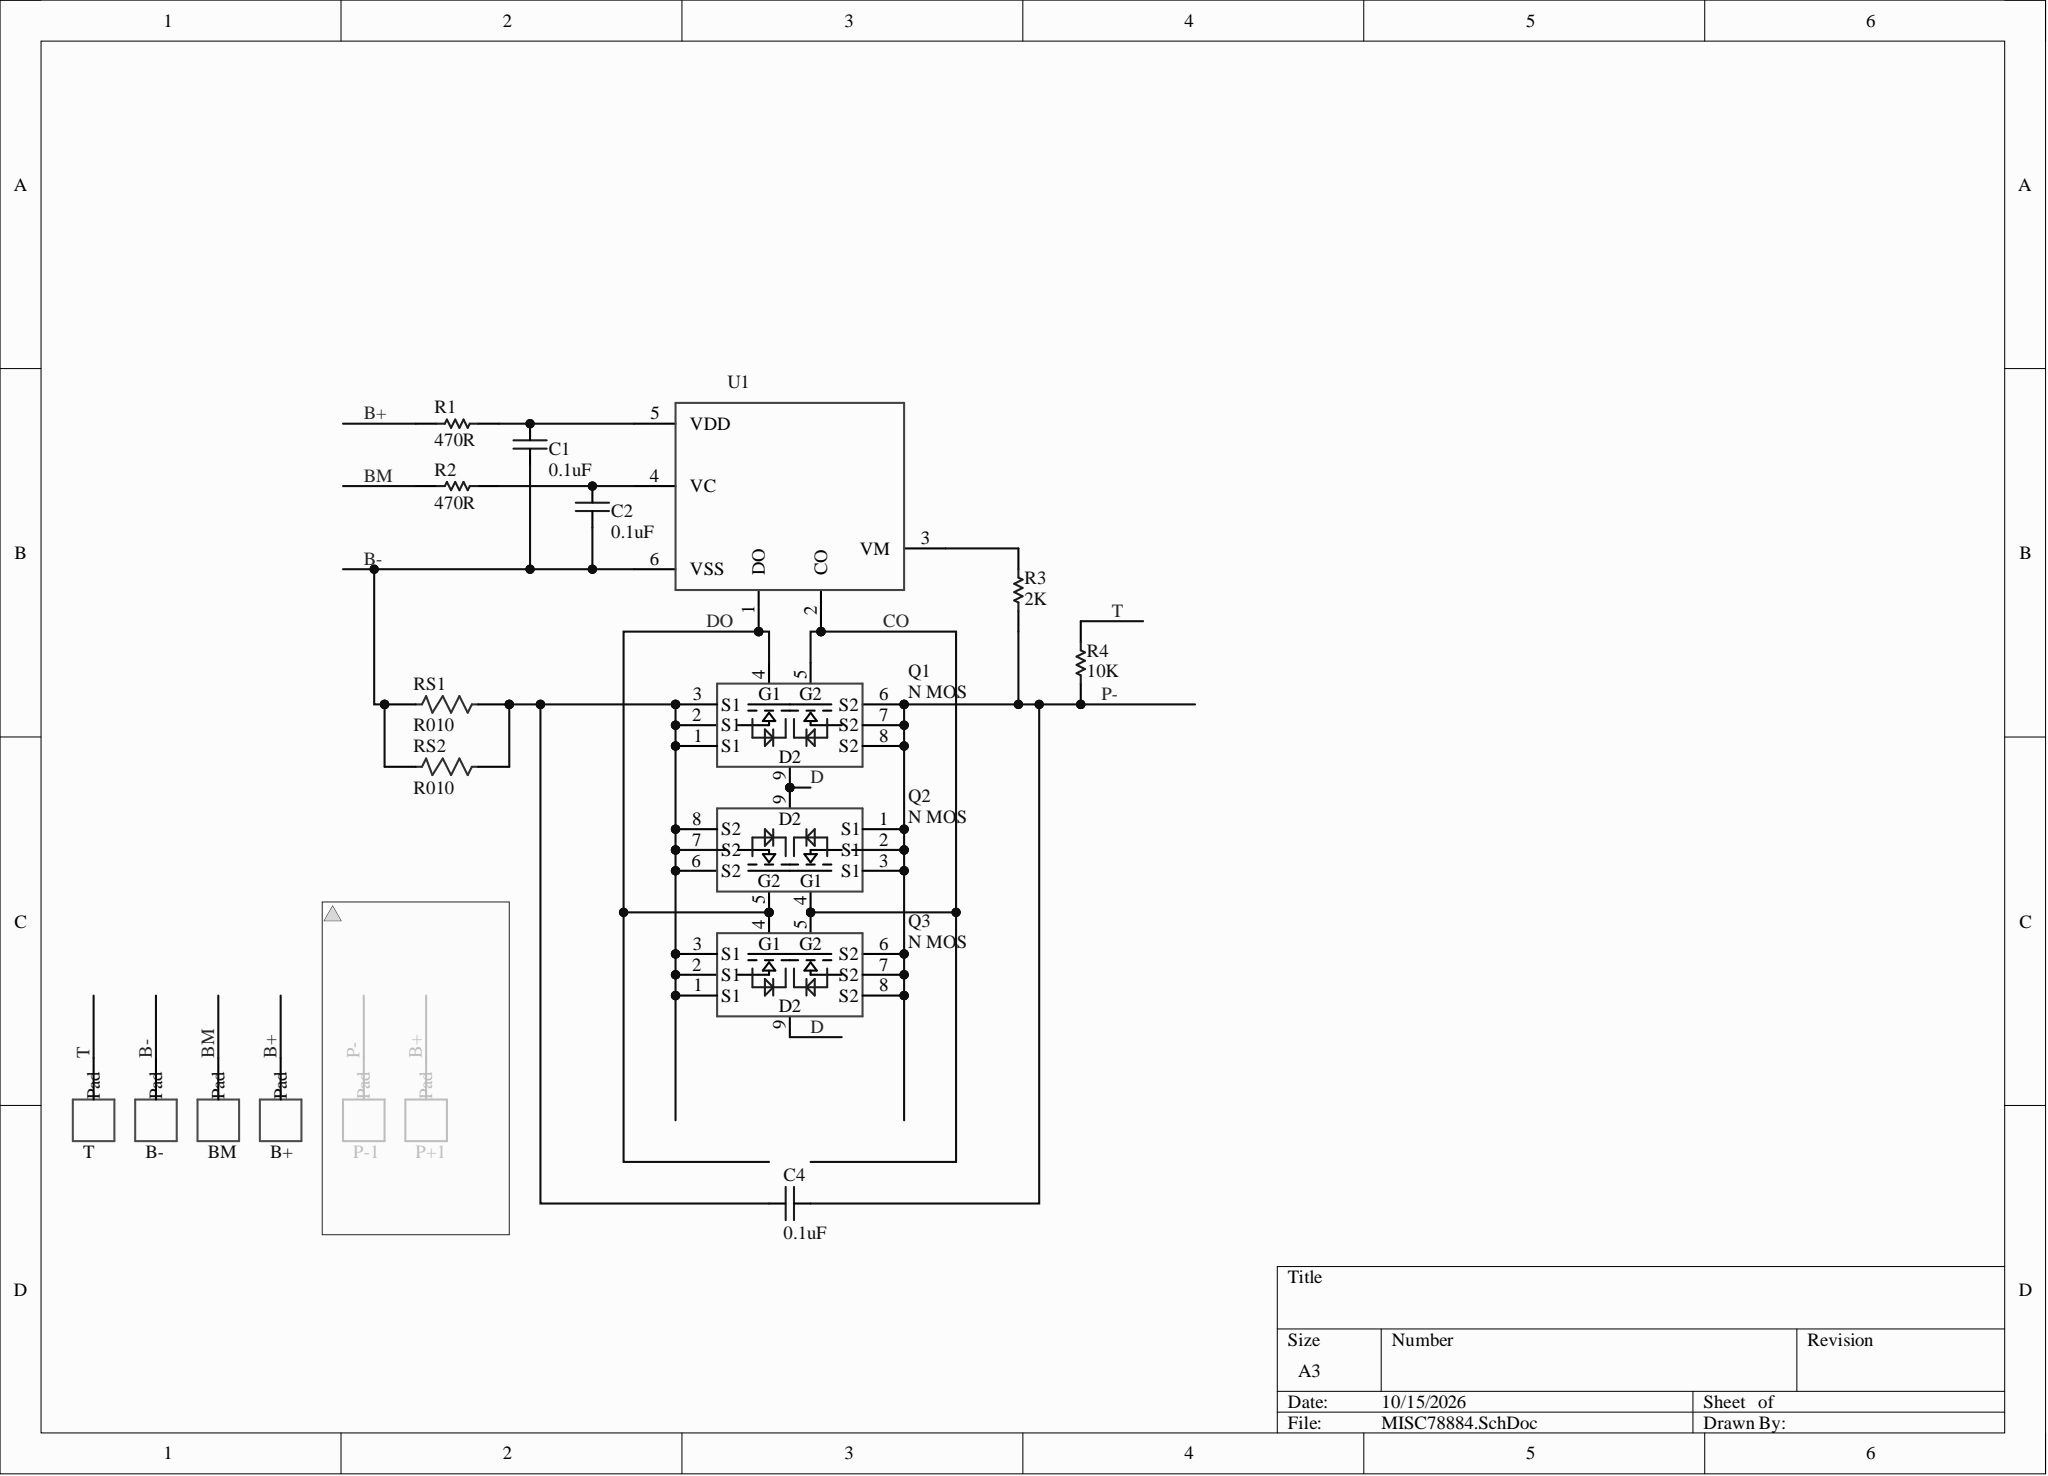Circuit board | Altium Designer | 17 parts | 12 nets
Bill of materials:
Comment,Description,Designator,Footprint,LibRef,Quantity
"Pad","Connection pad (non-through-hole)","B-, B+, BM, T","Pad10X8mm","Pad","4"
"0.1uF","SMD capacitor","C1, C2, C4","C0402A","CAP","3"
"N MOS","SMD MOS-TSSOP-8","Q1, Q2, Q3","DFN3*3-L8(2N)","2N MOS","3"
"470R","SMD resistor","R1, R2","R0402A","RES","2"
"2K","SMD resistor","R3","R0402A","RES","1"
"10K","SMD resistor","R4","R0402A","RES","1"
"R010","SMD alloy resistor","RS1, RS2","R2512L","RES2","2"
"","","U1","SOT23-6A","S-8252","1"
Netlist (Protel format):
[
B+
Pad10X8mm
Pad



]
[
B-
Pad10X8mm
Pad



]
[
BM
Pad10X8mm
Pad



]
[
C1
C0402A
0.1uF



]
[
C2
C0402A
0.1uF



]
[
C4
C0402A
0.1uF



]
[
Q1
DFN3*3-L8(2N)
N MOS



]
[
Q2
DFN3*3-L8(2N)
N MOS



]
[
Q3
DFN3*3-L8(2N)
N MOS



]
[
R1
R0402A
470R



]
[
R2
R0402A
470R



]
[
R3
R0402A
2K



]
[
R4
R0402A
10K



]
[
RS1
R2512L
R010



]
[
RS2
R2512L
R010



]
[
T
Pad10X8mm
Pad



]
[
U1
SOT23-6A




]
(
T
R4-2
T-1
)
(
P-
C4-1
Q1-6
Q1-7
Q1-8
Q2-1
Q2-2
Q2-3
Q3-6
Q3-7
Q3-8
R3-1
R4-1
)
(
NetR3_2
R3-2
U1-3
)
(
NetC4_2
C4-2
Q1-1
Q1-2
Q1-3
Q2-6
Q2-7
Q2-8
Q3-1
Q3-2
Q3-3
RS1-2
RS2-2
)
(
NetC2_2
C2-2
R2-2
U1-4
)
(
NetC1_2
C1-2
R1-2
U1-5
)
(
DO
Q1-4
Q2-5
Q3-4
U1-1
)
(
D
Q1-9
Q2-9
Q3-9
)
(
CO
Q1-5
Q2-4
Q3-5
U1-2
)
(
BM
BM-1
R2-1
)
(
B-
B--1
C1-1
C2-1
RS1-1
RS2-1
U1-6
)
(
B+
B+-1
R1-1
)